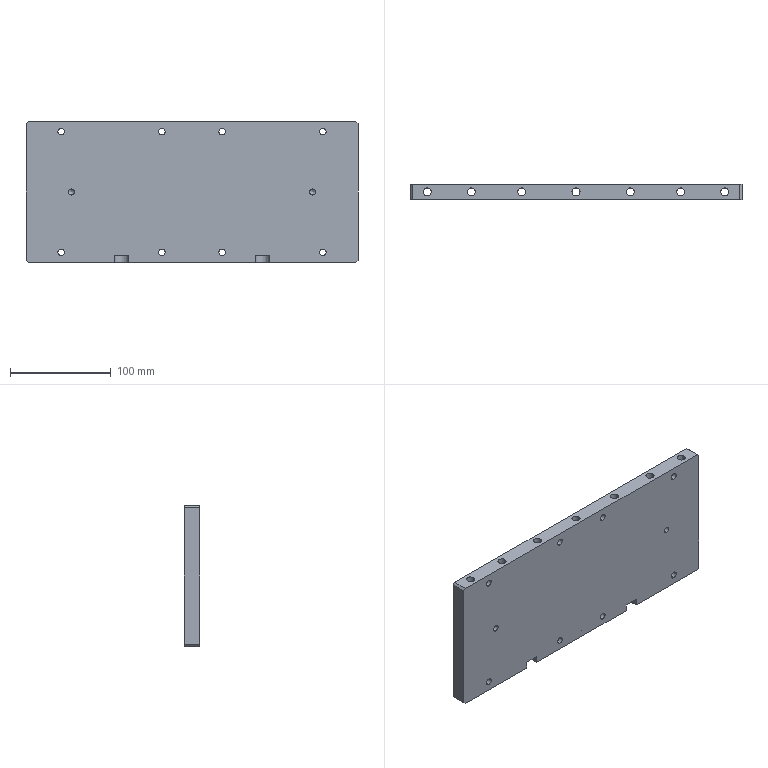Part | SolidWorks | features BaseBody 1 | 1 solid | 166 faces | box 330 x 15 x 140 mm | volume 621022 mm3 | cylinder 103 | plane 33 | cone 30 | commonest cylinder face diameters 8 x24 6.6 x16 11 x16 3.3 x14 6 x12 13 x11